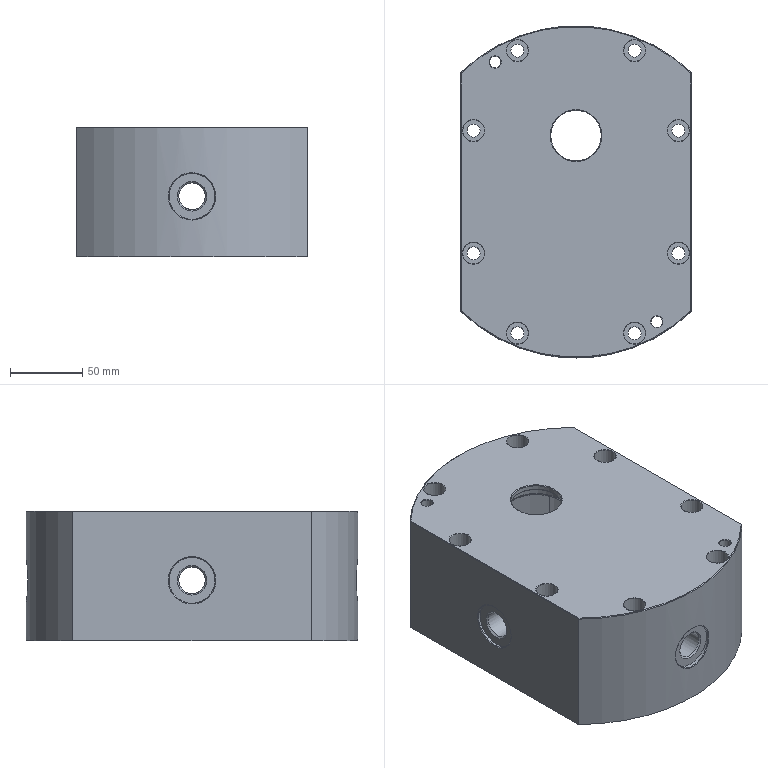NC program | NX | posted with a generic post | part box 160 x 230 x 90 mm
Whole program:
N10 G17 G21 G94 G90
(HOLE_MILLING_COPY_2 , TOOL : D10)
N12 T10 M6
N14 G54
N16 G17 G0 G90 X0. Y3. B0. C0. S3000 M3
N18 G43 Z30. H10
N20 Z0.624
N22 G94 G3 X-1.817 Y4.817 R1.817 F2200.
N24 X-3.633 Y3. R1.817
N26 X-3.633 Y3. Z0.404 I3.633 J0.
N28 X-3.633 Y3. Z0.184 I3.633 J0.
N30 X-3.633 Y3. Z-0.036 I3.633 J0.
N32 X-3.633 Y3. Z-0.256 I3.633 J0.
N34 X-3.633 Y3. Z-0.476 I3.633 J0.
N36 X-3.633 Y3. Z-0.696 I3.633 J0.
N38 X-3.633 Y3. Z-0.916 I3.633 J0.
N40 X-3.633 Y3. Z-1.136 I3.633 J0.
N42 X-3.633 Y3. Z-1.356 I3.633 J0.
N44 X-3.633 Y3. Z-1.576 I3.633 J0.
N46 X-3.633 Y3. Z-1.796 I3.633 J0.
N48 X-3.633 Y3. Z-2.016 I3.633 J0.
N50 X-3.633 Y3. Z-2.236 I3.633 J0.
N52 X-3.633 Y3. Z-2.456 I3.633 J0.
N54 X-3.633 Y3. Z-2.676 I3.633 J0.
N56 X-3.633 Y3. Z-2.896 I3.633 J0.
N58 X3.578 Y2.369 Z-3. R3.633
N60 X0.631 Y6.578 R3.633
N62 X3.578 Y2.369 R-3.633
N64 X2.105 Y4.473 R1.817
N66 X0. Y3. R1.817
N68 G0 Z0.624
N70 G3 X-3.633 Y6.633 R3.633
N72 X-7.267 Y3. R3.633
N74 X-7.267 Y3. Z0.404 I7.267 J0.
N76 X-7.267 Y3. Z0.184 I7.267 J0.
N78 X-7.267 Y3. Z-0.036 I7.267 J0.
N80 X-7.267 Y3. Z-0.256 I7.267 J0.
N82 X-7.267 Y3. Z-0.476 I7.267 J0.
N84 X-7.267 Y3. Z-0.696 I7.267 J0.
N86 X-7.267 Y3. Z-0.916 I7.267 J0.
N88 X-7.267 Y3. Z-1.136 I7.267 J0.
N90 X-7.267 Y3. Z-1.356 I7.267 J0.
N92 X-7.267 Y3. Z-1.576 I7.267 J0.
N94 X-7.267 Y3. Z-1.796 I7.267 J0.
N96 X-7.267 Y3. Z-2.016 I7.267 J0.
N98 X-7.267 Y3. Z-2.236 I7.267 J0.
N100 X-7.267 Y3. Z-2.456 I7.267 J0.
N102 X-7.267 Y3. Z-2.676 I7.267 J0.
N104 X-7.267 Y3. Z-2.896 I7.267 J0.
N106 X7.156 Y1.738 Z-3. R7.267
N108 X1.262 Y10.156 R7.267
N110 X7.156 Y1.738 R-7.267
N112 X4.209 Y5.947 R3.633
N114 X0. Y3. R3.633
N116 G0 Z0.624
N118 G3 X-5.45 Y8.45 R5.45
N120 X-10.9 Y3. R5.45
N122 X-10.9 Y3. Z0.404 I10.9 J0.
N124 X-10.9 Y3. Z0.184 I10.9 J0.
N126 X-10.9 Y3. Z-0.036 I10.9 J0.
N128 X-10.9 Y3. Z-0.256 I10.9 J0.
N130 X-10.9 Y3. Z-0.476 I10.9 J0.
N132 X-10.9 Y3. Z-0.696 I10.9 J0.
N134 X-10.9 Y3. Z-0.916 I10.9 J0.
N136 X-10.9 Y3. Z-1.136 I10.9 J0.
N138 X-10.9 Y3. Z-1.356 I10.9 J0.
N140 X-10.9 Y3. Z-1.576 I10.9 J0.
N142 X-10.9 Y3. Z-1.796 I10.9 J0.
N144 X-10.9 Y3. Z-2.016 I10.9 J0.
N146 X-10.9 Y3. Z-2.236 I10.9 J0.
N148 X-10.9 Y3. Z-2.456 I10.9 J0.
N150 X-10.9 Y3. Z-2.676 I10.9 J0.
N152 X-10.9 Y3. Z-2.896 I10.9 J0.
N154 X10.734 Y1.107 Z-3. R10.9
N156 X1.893 Y13.734 R10.9
N158 X10.734 Y1.107 R-10.9
N160 X6.314 Y7.42 R5.45
N162 X0. Y3. R5.45
N164 G0 Z30.
(HOLE_MILLING_COPY_COPY_1 , TOOL : D10)
N166 Z-2.5
N168 G3 X-2.075 Y5.075 R2.075
N170 X-4.15 Y3. R2.075
N172 X-4.15 Y3. Z-2.72 I4.15 J0.
N174 X-4.15 Y3. Z-2.94 I4.15 J0.
N176 X-4.15 Y3. Z-3.16 I4.15 J0.
N178 X-4.15 Y3. Z-3.38 I4.15 J0.
N180 X-4.15 Y3. Z-3.6 I4.15 J0.
N182 X-4.15 Y3. Z-3.82 I4.15 J0.
N184 X-4.15 Y3. Z-4.04 I4.15 J0.
N186 X-4.15 Y3. Z-4.26 I4.15 J0.
N188 X-4.15 Y3. Z-4.48 I4.15 J0.
N190 X-4.15 Y3. Z-4.7 I4.15 J0.
N192 X-4.15 Y3. Z-4.92 I4.15 J0.
N194 X-4.15 Y3. Z-5.14 I4.15 J0.
N196 X-4.15 Y3. Z-5.36 I4.15 J0.
N198 X-4.15 Y3. Z-5.58 I4.15 J0.
N200 X-4.15 Y3. Z-5.8 I4.15 J0.
N202 X-4.15 Y3. Z-6.02 I4.15 J0.
N204 X-4.15 Y3. Z-6.24 I4.15 J0.
N206 X-4.15 Y3. Z-6.46 I4.15 J0.
N208 X-4.15 Y3. Z-6.68 I4.15 J0.
N210 X-4.15 Y3. Z-6.9 I4.15 J0.
N212 X-4.15 Y3. Z-7.12 I4.15 J0.
N214 X-4.15 Y3. Z-7.34 I4.15 J0.
N216 X-4.15 Y3. Z-7.56 I4.15 J0.
N218 X-4.15 Y3. Z-7.78 I4.15 J0.
N220 X-4.15 Y3. Z-8. I4.15 J0.
N222 X-4.15 Y3. Z-8.22 I4.15 J0.
N224 X-4.15 Y3. Z-8.44 I4.15 J0.
N226 X-4.15 Y3. Z-8.66 I4.15 J0.
N228 X-4.15 Y3. Z-8.88 I4.15 J0.
N230 X-4.15 Y3. Z-9.1 I4.15 J0.
N232 X-4.15 Y3. Z-9.32 I4.15 J0.
N234 X-4.15 Y3. Z-9.54 I4.15 J0.
N236 X-4.15 Y3. Z-9.76 I4.15 J0.
N238 X-4.15 Y3. Z-9.98 I4.15 J0.
N240 X-4.15 Y3. Z-10.2 I4.15 J0.
N242 X-4.15 Y3. Z-10.42 I4.15 J0.
N244 X-4.15 Y3. Z-10.64 I4.15 J0.
N246 X-4.15 Y3. Z-10.86 I4.15 J0.
N248 X-4.15 Y3. Z-11.08 I4.15 J0.
N250 X-4.15 Y3. Z-11.3 I4.15 J0.
N252 X-4.15 Y3. Z-11.52 I4.15 J0.
N254 X-4.15 Y3. Z-11.74 I4.15 J0.
N256 X-4.15 Y3. Z-11.96 I4.15 J0.
N258 X-4.15 Y3. Z-12.18 I4.15 J0.
N260 X-4.15 Y3. Z-12.4 I4.15 J0.
N262 X-4.15 Y3. Z-12.62 I4.15 J0.
N264 X-4.15 Y3. Z-12.84 I4.15 J0.
N266 X-4.15 Y3. Z-13.06 I4.15 J0.
N268 X-4.15 Y3. Z-13.28 I4.15 J0.
N270 X-4.15 Y3. Z-13.5 I4.15 J0.
N272 X-4.15 Y3. Z-13.72 I4.15 J0.
N274 X-4.15 Y3. Z-13.94 I4.15 J0.
N276 X-4.15 Y3. Z-14.16 I4.15 J0.
N278 X-4.15 Y3. Z-14.38 I4.15 J0.
N280 X-4.15 Y3. Z-14.6 I4.15 J0.
N282 X-4.15 Y3. Z-14.82 I4.15 J0.
N284 X-4.15 Y3. Z-15.04 I4.15 J0.
N286 X-4.15 Y3. Z-15.26 I4.15 J0.
N288 X-4.15 Y3. Z-15.48 I4.15 J0.
N290 X-4.15 Y3. Z-15.7 I4.15 J0.
N292 X-4.15 Y3. Z-15.92 I4.15 J0.
N294 X-4.15 Y3. Z-16.14 I4.15 J0.
N296 X-4.15 Y3. Z-16.36 I4.15 J0.
N298 X-4.15 Y3. Z-16.58 I4.15 J0.
N300 X-4.15 Y3. Z-16.8 I4.15 J0.
N302 X-4.15 Y3. Z-17.02 I4.15 J0.
N304 X-4.15 Y3. Z-17.24 I4.15 J0.
N306 X-4.15 Y3. Z-17.46 I4.15 J0.
N308 X-4.15 Y3. Z-17.68 I4.15 J0.
N310 X-4.15 Y3. Z-17.9 I4.15 J0.
N312 X-4.15 Y3. Z-18.12 I4.15 J0.
N314 X-4.15 Y3. Z-18.34 I4.15 J0.
N316 X-4.15 Y3. Z-18.56 I4.15 J0.
N318 X-4.15 Y3. Z-18.78 I4.15 J0.
N320 X-4.15 Y3. Z-19. I4.15 J0.
N322 X-4.15 Y3. Z-19.22 I4.15 J0.
N324 X-4.15 Y3. Z-19.44 I4.15 J0.
N326 X-4.15 Y3. Z-19.66 I4.15 J0.
N328 X-4.15 Y3. Z-19.88 I4.15 J0.
N330 X-4.15 Y3. Z-20.1 I4.15 J0.
N332 X-4.15 Y3. Z-20.32 I4.15 J0.
N334 X-4.15 Y3. Z-20.54 I4.15 J0.
N336 X-4.15 Y3. Z-20.76 I4.15 J0.
N338 X-4.15 Y3. Z-20.98 I4.15 J0.
N340 X-4.15 Y3. Z-21.2 I4.15 J0.
N342 X-4.15 Y3. Z-21.42 I4.15 J0.
N344 X-4.15 Y3. Z-21.64 I4.15 J0.
N346 X-4.15 Y3. Z-21.86 I4.15 J0.
N348 X-4.15 Y3. Z-22.08 I4.15 J0.
N350 X-4.15 Y3. Z-22.3 I4.15 J0.
N352 X0.455 Y7.125 Z-22.461 R-4.15
N354 X-4.125 Y3.455 R4.15
N356 X0.455 Y7.125 R-4.15
N358 X-1.835 Y5.29 R2.075
N360 X0. Y3. R2.075
N362 G0 Z30.
N364 M5
(HOLE_MILLING_COPY_1_COPY_2 , TOOL : D10JING)
N366 T11 M6
N368 G54
N370 G17 G0 G90 X0. Y3. B0. C0. S5000 M3
N372 G43 Z30. H11
N374 Z-3.
N376 G94 G1 X-7.486 Y5.524 F1000.
N378 G3 X-11. Y3. R2.663
N380 X0. Y-8. R11.
N382 X-11. Y3. R-11.
N384 X-7.486 Y0.476 R2.663
N386 G1 X0. Y3.
N388 G0 Z30.
(HOLE_MILLING_COPY_1_COPY_COPY , TOOL : D10JING)
N390 Z-22.461
N392 G1 X-0.58 Y3.993
N394 G3 X-4.25 Y3. R1.969
N396 X0. Y-1.25 R4.25
N398 X-4.25 Y3. R-4.25
N400 X-0.58 Y2.007 R1.969
N402 G1 X0. Y3.
N404 G0 Z30.
N406 M5
(PLANAR_MILL_COPY_COPY_COPY_1 , TOOL : D6A45)
N408 T07 M6
N410 G54
N412 G17 G0 G90 X1.621 Y10.374 B0. C0. S7500 M3
N414 G43 Z30. H7
N416 Z-1.5
N418 G94 G1 Z-4.5 F1250.
N420 X0.766 Y11.393
N422 G3 X0. Y11.75 R1.
N424 X-8.75 Y3. R8.75
N426 X0. Y11.75 R-8.75
N428 X-0.766 Y11.393 R1.
N430 G1 X-1.621 Y10.374
N432 Z-1.5
N434 G0 Z30.
(PROFILE_3D , TOOL : D6A45)
N436 X-1.067 Y-10.742
N438 Z1.609
N440 G1 Z-1.391
N442 X-0.531 Y-11.672
N444 G3 X-0.011 Y-11.973 R0.6
N446 G1 X0.863 Z-1.401
N448 X2.597 Y-11.772 Z-1.42
N450 X4.295 Y-11.369 Z-1.509
N452 X5.936 Y-10.773 Z-1.597
N454 X7.496 Y-9.99 Z-1.686
N456 X8.953 Y-9.033 Z-1.807
N458 X10.289 Y-7.914 Z-1.927
N460 X11.513 Y-6.613 Z-2.051
N462 X12.574 Y-5.176 Z-2.175
N464 X13.457 Y-3.623 Z-2.298
N466 X14.15 Y-1.975 Z-2.422
N468 X14.641 Y-0.256 Z-2.485
N470 X14.925 Y1.51 Z-2.548
N472 X14.995 Y3.297 Z-2.559
N474 X14.853 Y5.081 Z-2.52
N476 X14.499 Y6.836 Z-2.48
N478 X13.94 Y8.535 Z-2.371
N480 X13.182 Y10.155 Z-2.262
N482 X12.238 Y11.672 Z-2.153
N484 X11.12 Y13.065 Z-2.027
N486 X9.845 Y14.315 Z-1.9
N488 X8.429 Y15.405 Z-1.774
N490 X6.893 Y16.32 Z-1.648
N492 X5.258 Y17.046 Z-1.521
N494 X3.548 Y17.573 Z-1.457
N496 X1.787 Y17.892 Z-1.392
N498 X-0.005 Y17.999 Z-1.403
N500 X-1.472 Y17.927 Z-1.413
N502 X-2.929 Y17.711 Z-1.422
N504 X-4.358 Y17.353 Z-1.499
N506 X-5.743 Y16.857 Z-1.575
N508 X-7.072 Y16.228 Z-1.652
N510 X-8.334 Y15.471 Z-1.759
N512 X-9.515 Y14.595 Z-1.866
N514 X-10.605 Y13.607 Z-1.974
N516 X-11.592 Y12.517 Z-2.081
N518 X-12.466 Y11.339 Z-2.188
N520 X-13.342 Y9.85 Z-2.314
N522 X-14.04 Y8.273 Z-2.386
N524 X-14.552 Y6.625 Z-2.458
N526 X-14.872 Y4.929 Z-2.529
N528 X-14.995 Y3.206 Z-2.535
N530 X-14.92 Y1.481 Z-2.541
N532 X-14.647 Y-0.223 Z-2.474
N534 X-14.18 Y-1.886 Z-2.408
N536 X-13.583 Y-3.364 Z-2.346
N538 X-12.831 Y-4.771 Z-2.23
N540 X-11.934 Y-6.089 Z-2.115
N542 X-10.904 Y-7.304 Z-1.999
N544 X-9.75 Y-8.402 Z-1.884
N546 X-8.486 Y-9.371 Z-1.769
N548 X-7.125 Y-10.201 Z-1.653
N550 X-5.682 Y-10.882 Z-1.538
N552 X-4.174 Y-11.406 Z-1.487
N554 X-2.621 Y-11.767 Z-1.437
N556 X-0.884 Y-11.972 Z-1.381
N558 X-0.011 Y-11.973 Z-1.391
N560 G3 X0.509 Y-11.673 R0.6
N562 G1 X1.046 Y-10.744
N564 Z1.609
N566 G0 Z30.
N568 M5
N570 M2